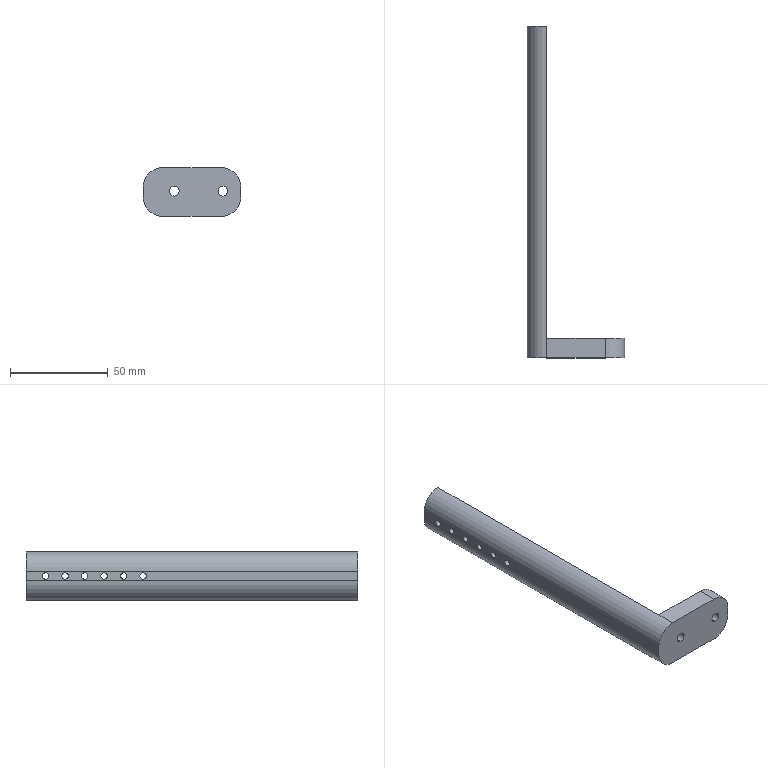Part | STEP file | L.step.STEP.STEP-181.STEP | 1 solid | 28 faces | box 50 x 170 x 25 mm | volume 43868 mm3 | cylinder 20 | plane 8 | commonest cylinder face diameters 3.3 x12 5 x4 20 x4
STEP:
#1=CARTESIAN_POINT('',(96.633,122.7,-36.277));
#2=VERTEX_POINT('',#1);
#3=CARTESIAN_POINT('',(96.633,122.7,-39.577));
#4=VERTEX_POINT('',#3);
#5=CARTESIAN_POINT('',(96.633,122.7,-37.927));
#6=DIRECTION('',(1.,0.,0.));
#7=DIRECTION('',(0.,0.,-1.));
#8=AXIS2_PLACEMENT_3D('',#5,#6,#7);
#9=CIRCLE('',#8,1.65);
#10=EDGE_CURVE('',#2,#4,#9,.T.);
#11=ORIENTED_EDGE('',*,*,#10,.F.);
#12=CARTESIAN_POINT('',(106.633,122.7,-36.277));
#13=VERTEX_POINT('',#12);
#14=CARTESIAN_POINT('',(106.633,122.7,-36.277));
#15=DIRECTION('',(1.,0.,0.));
#16=VECTOR('',#15,1000.);
#17=LINE('',#14,#16);
#18=EDGE_CURVE('',#2,#13,#17,.T.);
#19=ORIENTED_EDGE('',*,*,#18,.T.);
#20=CARTESIAN_POINT('',(106.633,122.7,-39.577));
#21=VERTEX_POINT('',#20);
#22=CARTESIAN_POINT('',(106.633,122.7,-37.927));
#23=DIRECTION('',(1.,0.,0.));
#24=DIRECTION('',(0.,0.,-1.));
#25=AXIS2_PLACEMENT_3D('',#22,#23,#24);
#26=CIRCLE('',#25,1.65);
#27=EDGE_CURVE('',#13,#21,#26,.T.);
#28=ORIENTED_EDGE('',*,*,#27,.T.);
#29=CARTESIAN_POINT('',(106.633,122.7,-39.577));
#30=DIRECTION('',(1.,0.,0.));
#31=VECTOR('',#30,1000.);
#32=LINE('',#29,#31);
#33=EDGE_CURVE('',#4,#21,#32,.T.);
#34=ORIENTED_EDGE('',*,*,#33,.F.);
#35=EDGE_LOOP('',(#11,#19,#28,#34));
#36=FACE_OUTER_BOUND('',#35,.T.);
#37=CARTESIAN_POINT('',(106.633,122.7,-37.927));
#38=DIRECTION('',(1.,0.,0.));
#39=DIRECTION('',(0.,0.,-1.));
#40=AXIS2_PLACEMENT_3D('',#37,#38,#39);
#41=CYLINDRICAL_SURFACE('',#40,1.65);
#42=ADVANCED_FACE('',(#36),#41,.F.);
#43=CARTESIAN_POINT('',(96.633,132.7,-36.277));
#44=VERTEX_POINT('',#43);
#45=CARTESIAN_POINT('',(96.633,132.7,-39.577));
#46=VERTEX_POINT('',#45);
#47=CARTESIAN_POINT('',(96.633,132.7,-37.927));
#48=DIRECTION('',(1.,0.,0.));
#49=DIRECTION('',(0.,0.,-1.));
#50=AXIS2_PLACEMENT_3D('',#47,#48,#49);
#51=CIRCLE('',#50,1.65);
#52=EDGE_CURVE('',#44,#46,#51,.T.);
#53=ORIENTED_EDGE('',*,*,#52,.F.);
#54=CARTESIAN_POINT('',(106.633,132.7,-36.277));
#55=VERTEX_POINT('',#54);
#56=CARTESIAN_POINT('',(106.633,132.7,-36.277));
#57=DIRECTION('',(1.,0.,0.));
#58=VECTOR('',#57,1000.);
#59=LINE('',#56,#58);
#60=EDGE_CURVE('',#44,#55,#59,.T.);
#61=ORIENTED_EDGE('',*,*,#60,.T.);
#62=CARTESIAN_POINT('',(106.633,132.7,-39.577));
#63=VERTEX_POINT('',#62);
#64=CARTESIAN_POINT('',(106.633,132.7,-37.927));
#65=DIRECTION('',(1.,0.,0.));
#66=DIRECTION('',(0.,0.,-1.));
#67=AXIS2_PLACEMENT_3D('',#64,#65,#66);
#68=CIRCLE('',#67,1.65);
#69=EDGE_CURVE('',#55,#63,#68,.T.);
#70=ORIENTED_EDGE('',*,*,#69,.T.);
#71=CARTESIAN_POINT('',(106.633,132.7,-39.577));
#72=DIRECTION('',(1.,0.,0.));
#73=VECTOR('',#72,1000.);
#74=LINE('',#71,#73);
#75=EDGE_CURVE('',#46,#63,#74,.T.);
#76=ORIENTED_EDGE('',*,*,#75,.F.);
#77=EDGE_LOOP('',(#53,#61,#70,#76));
#78=FACE_OUTER_BOUND('',#77,.T.);
#79=CARTESIAN_POINT('',(106.633,132.7,-37.927));
#80=DIRECTION('',(1.,0.,0.));
#81=DIRECTION('',(0.,0.,-1.));
#82=AXIS2_PLACEMENT_3D('',#79,#80,#81);
#83=CYLINDRICAL_SURFACE('',#82,1.65);
#84=ADVANCED_FACE('',(#78),#83,.F.);
#85=CARTESIAN_POINT('',(96.633,142.7,-36.277));
#86=VERTEX_POINT('',#85);
#87=CARTESIAN_POINT('',(96.633,142.7,-39.577));
#88=VERTEX_POINT('',#87);
#89=CARTESIAN_POINT('',(96.633,142.7,-37.927));
#90=DIRECTION('',(1.,0.,0.));
#91=DIRECTION('',(0.,0.,-1.));
#92=AXIS2_PLACEMENT_3D('',#89,#90,#91);
#93=CIRCLE('',#92,1.65);
#94=EDGE_CURVE('',#86,#88,#93,.T.);
#95=ORIENTED_EDGE('',*,*,#94,.F.);
#96=CARTESIAN_POINT('',(106.633,142.7,-36.277));
#97=VERTEX_POINT('',#96);
#98=CARTESIAN_POINT('',(106.633,142.7,-36.277));
#99=DIRECTION('',(1.,0.,0.));
#100=VECTOR('',#99,1000.);
#101=LINE('',#98,#100);
#102=EDGE_CURVE('',#86,#97,#101,.T.);
#103=ORIENTED_EDGE('',*,*,#102,.T.);
#104=CARTESIAN_POINT('',(106.633,142.7,-39.577));
#105=VERTEX_POINT('',#104);
#106=CARTESIAN_POINT('',(106.633,142.7,-37.927));
#107=DIRECTION('',(1.,0.,0.));
#108=DIRECTION('',(0.,0.,-1.));
#109=AXIS2_PLACEMENT_3D('',#106,#107,#108);
#110=CIRCLE('',#109,1.65);
#111=EDGE_CURVE('',#97,#105,#110,.T.);
#112=ORIENTED_EDGE('',*,*,#111,.T.);
#113=CARTESIAN_POINT('',(106.633,142.7,-39.577));
#114=DIRECTION('',(1.,0.,0.));
#115=VECTOR('',#114,1000.);
#116=LINE('',#113,#115);
#117=EDGE_CURVE('',#88,#105,#116,.T.);
#118=ORIENTED_EDGE('',*,*,#117,.F.);
#119=EDGE_LOOP('',(#95,#103,#112,#118));
#120=FACE_OUTER_BOUND('',#119,.T.);
#121=CARTESIAN_POINT('',(106.633,142.7,-37.927));
#122=DIRECTION('',(1.,0.,0.));
#123=DIRECTION('',(0.,0.,-1.));
#124=AXIS2_PLACEMENT_3D('',#121,#122,#123);
#125=CYLINDRICAL_SURFACE('',#124,1.65);
#126=ADVANCED_FACE('',(#120),#125,.F.);
#127=CARTESIAN_POINT('',(96.633,152.7,-36.277));
#128=VERTEX_POINT('',#127);
#129=CARTESIAN_POINT('',(96.633,152.7,-39.577));
#130=VERTEX_POINT('',#129);
#131=CARTESIAN_POINT('',(96.633,152.7,-37.927));
#132=DIRECTION('',(1.,0.,0.));
#133=DIRECTION('',(0.,0.,-1.));
#134=AXIS2_PLACEMENT_3D('',#131,#132,#133);
#135=CIRCLE('',#134,1.65);
#136=EDGE_CURVE('',#128,#130,#135,.T.);
#137=ORIENTED_EDGE('',*,*,#136,.F.);
#138=CARTESIAN_POINT('',(106.633,152.7,-36.277));
#139=VERTEX_POINT('',#138);
#140=CARTESIAN_POINT('',(106.633,152.7,-36.277));
#141=DIRECTION('',(1.,0.,0.));
#142=VECTOR('',#141,1000.);
#143=LINE('',#140,#142);
#144=EDGE_CURVE('',#128,#139,#143,.T.);
#145=ORIENTED_EDGE('',*,*,#144,.T.);
#146=CARTESIAN_POINT('',(106.633,152.7,-39.577));
#147=VERTEX_POINT('',#146);
#148=CARTESIAN_POINT('',(106.633,152.7,-37.927));
#149=DIRECTION('',(1.,0.,0.));
#150=DIRECTION('',(0.,0.,-1.));
#151=AXIS2_PLACEMENT_3D('',#148,#149,#150);
#152=CIRCLE('',#151,1.65);
#153=EDGE_CURVE('',#139,#147,#152,.T.);
#154=ORIENTED_EDGE('',*,*,#153,.T.);
#155=CARTESIAN_POINT('',(106.633,152.7,-39.577));
#156=DIRECTION('',(1.,0.,0.));
#157=VECTOR('',#156,1000.);
#158=LINE('',#155,#157);
#159=EDGE_CURVE('',#130,#147,#158,.T.);
#160=ORIENTED_EDGE('',*,*,#159,.F.);
#161=EDGE_LOOP('',(#137,#145,#154,#160));
#162=FACE_OUTER_BOUND('',#161,.T.);
#163=CARTESIAN_POINT('',(106.633,152.7,-37.927));
#164=DIRECTION('',(1.,0.,0.));
#165=DIRECTION('',(0.,0.,-1.));
#166=AXIS2_PLACEMENT_3D('',#163,#164,#165);
#167=CYLINDRICAL_SURFACE('',#166,1.65);
#168=ADVANCED_FACE('',(#162),#167,.F.);
#169=CARTESIAN_POINT('',(96.633,162.7,-36.277));
#170=VERTEX_POINT('',#169);
#171=CARTESIAN_POINT('',(96.633,162.7,-39.577));
#172=VERTEX_POINT('',#171);
#173=CARTESIAN_POINT('',(96.633,162.7,-37.927));
#174=DIRECTION('',(1.,0.,0.));
#175=DIRECTION('',(0.,0.,-1.));
#176=AXIS2_PLACEMENT_3D('',#173,#174,#175);
#177=CIRCLE('',#176,1.65);
#178=EDGE_CURVE('',#170,#172,#177,.T.);
#179=ORIENTED_EDGE('',*,*,#178,.F.);
#180=CARTESIAN_POINT('',(106.633,162.7,-36.277));
#181=VERTEX_POINT('',#180);
#182=CARTESIAN_POINT('',(106.633,162.7,-36.277));
#183=DIRECTION('',(1.,0.,0.));
#184=VECTOR('',#183,1000.);
#185=LINE('',#182,#184);
#186=EDGE_CURVE('',#170,#181,#185,.T.);
#187=ORIENTED_EDGE('',*,*,#186,.T.);
#188=CARTESIAN_POINT('',(106.633,162.7,-39.577));
#189=VERTEX_POINT('',#188);
#190=CARTESIAN_POINT('',(106.633,162.7,-37.927));
#191=DIRECTION('',(1.,0.,0.));
#192=DIRECTION('',(0.,0.,-1.));
#193=AXIS2_PLACEMENT_3D('',#190,#191,#192);
#194=CIRCLE('',#193,1.65);
#195=EDGE_CURVE('',#181,#189,#194,.T.);
#196=ORIENTED_EDGE('',*,*,#195,.T.);
#197=CARTESIAN_POINT('',(106.633,162.7,-39.577));
#198=DIRECTION('',(1.,0.,0.));
#199=VECTOR('',#198,1000.);
#200=LINE('',#197,#199);
#201=EDGE_CURVE('',#172,#189,#200,.T.);
#202=ORIENTED_EDGE('',*,*,#201,.F.);
#203=EDGE_LOOP('',(#179,#187,#196,#202));
#204=FACE_OUTER_BOUND('',#203,.T.);
#205=CARTESIAN_POINT('',(106.633,162.7,-37.927));
#206=DIRECTION('',(1.,0.,0.));
#207=DIRECTION('',(0.,0.,-1.));
#208=AXIS2_PLACEMENT_3D('',#205,#206,#207);
#209=CYLINDRICAL_SURFACE('',#208,1.65);
#210=ADVANCED_FACE('',(#204),#209,.F.);
#211=CARTESIAN_POINT('',(96.633,172.7,-36.277));
#212=VERTEX_POINT('',#211);
#213=CARTESIAN_POINT('',(96.633,172.7,-39.577));
#214=VERTEX_POINT('',#213);
#215=CARTESIAN_POINT('',(96.633,172.7,-37.927));
#216=DIRECTION('',(1.,0.,0.));
#217=DIRECTION('',(0.,0.,-1.));
#218=AXIS2_PLACEMENT_3D('',#215,#216,#217);
#219=CIRCLE('',#218,1.65);
#220=EDGE_CURVE('',#212,#214,#219,.T.);
#221=ORIENTED_EDGE('',*,*,#220,.F.);
#222=CARTESIAN_POINT('',(106.633,172.7,-36.277));
#223=VERTEX_POINT('',#222);
#224=CARTESIAN_POINT('',(106.633,172.7,-36.277));
#225=DIRECTION('',(1.,0.,0.));
#226=VECTOR('',#225,1000.);
#227=LINE('',#224,#226);
#228=EDGE_CURVE('',#212,#223,#227,.T.);
#229=ORIENTED_EDGE('',*,*,#228,.T.);
#230=CARTESIAN_POINT('',(106.633,172.7,-39.577));
#231=VERTEX_POINT('',#230);
#232=CARTESIAN_POINT('',(106.633,172.7,-37.927));
#233=DIRECTION('',(1.,0.,0.));
#234=DIRECTION('',(0.,0.,-1.));
#235=AXIS2_PLACEMENT_3D('',#232,#233,#234);
#236=CIRCLE('',#235,1.65);
#237=EDGE_CURVE('',#223,#231,#236,.T.);
#238=ORIENTED_EDGE('',*,*,#237,.T.);
#239=CARTESIAN_POINT('',(106.633,172.7,-39.577));
#240=DIRECTION('',(1.,0.,0.));
#241=VECTOR('',#240,1000.);
#242=LINE('',#239,#241);
#243=EDGE_CURVE('',#214,#231,#242,.T.);
#244=ORIENTED_EDGE('',*,*,#243,.F.);
#245=EDGE_LOOP('',(#221,#229,#238,#244));
#246=FACE_OUTER_BOUND('',#245,.T.);
#247=CARTESIAN_POINT('',(106.633,172.7,-37.927));
#248=DIRECTION('',(1.,0.,0.));
#249=DIRECTION('',(0.,0.,-1.));
#250=AXIS2_PLACEMENT_3D('',#247,#248,#249);
#251=CYLINDRICAL_SURFACE('',#250,1.65);
#252=ADVANCED_FACE('',(#246),#251,.F.);
#253=CARTESIAN_POINT('',(112.5,22.7,-35.));
#254=VERTEX_POINT('',#253);
#255=CARTESIAN_POINT('',(112.5,22.7,-40.));
#256=VERTEX_POINT('',#255);
#257=CARTESIAN_POINT('',(112.5,22.7,-37.5));
#258=DIRECTION('',(0.,-1.,0.));
#259=DIRECTION('',(0.,0.,-1.));
#260=AXIS2_PLACEMENT_3D('',#257,#258,#259);
#261=CIRCLE('',#260,2.5);
#262=EDGE_CURVE('',#254,#256,#261,.T.);
#263=ORIENTED_EDGE('',*,*,#262,.F.);
#264=CARTESIAN_POINT('',(112.5,12.7,-35.));
#265=VERTEX_POINT('',#264);
#266=CARTESIAN_POINT('',(112.5,0.,-35.));
#267=DIRECTION('',(0.,-1.,0.));
#268=VECTOR('',#267,1000.);
#269=LINE('',#266,#268);
#270=EDGE_CURVE('',#254,#265,#269,.T.);
#271=ORIENTED_EDGE('',*,*,#270,.T.);
#272=CARTESIAN_POINT('',(112.5,12.7,-40.));
#273=VERTEX_POINT('',#272);
#274=CARTESIAN_POINT('',(112.5,12.7,-37.5));
#275=DIRECTION('',(0.,1.,0.));
#276=DIRECTION('',(0.,0.,1.));
#277=AXIS2_PLACEMENT_3D('',#274,#275,#276);
#278=CIRCLE('',#277,2.5);
#279=EDGE_CURVE('',#273,#265,#278,.T.);
#280=ORIENTED_EDGE('',*,*,#279,.F.);
#281=CARTESIAN_POINT('',(112.5,0.,-40.));
#282=DIRECTION('',(0.,-1.,0.));
#283=VECTOR('',#282,1000.);
#284=LINE('',#281,#283);
#285=EDGE_CURVE('',#256,#273,#284,.T.);
#286=ORIENTED_EDGE('',*,*,#285,.F.);
#287=EDGE_LOOP('',(#263,#271,#280,#286));
#288=FACE_OUTER_BOUND('',#287,.T.);
#289=CARTESIAN_POINT('',(112.5,0.,-37.5));
#290=DIRECTION('',(0.,-1.,0.));
#291=DIRECTION('',(0.,0.,-1.));
#292=AXIS2_PLACEMENT_3D('',#289,#290,#291);
#293=CYLINDRICAL_SURFACE('',#292,2.5);
#294=ADVANCED_FACE('',(#288),#293,.F.);
#295=CARTESIAN_POINT('',(137.5,22.7,-35.));
#296=VERTEX_POINT('',#295);
#297=CARTESIAN_POINT('',(137.5,22.7,-40.));
#298=VERTEX_POINT('',#297);
#299=CARTESIAN_POINT('',(137.5,22.7,-37.5));
#300=DIRECTION('',(0.,-1.,0.));
#301=DIRECTION('',(0.,0.,-1.));
#302=AXIS2_PLACEMENT_3D('',#299,#300,#301);
#303=CIRCLE('',#302,2.5);
#304=EDGE_CURVE('',#296,#298,#303,.T.);
#305=ORIENTED_EDGE('',*,*,#304,.F.);
#306=CARTESIAN_POINT('',(137.5,12.7,-35.));
#307=VERTEX_POINT('',#306);
#308=CARTESIAN_POINT('',(137.5,0.,-35.));
#309=DIRECTION('',(0.,-1.,0.));
#310=VECTOR('',#309,1000.);
#311=LINE('',#308,#310);
#312=EDGE_CURVE('',#296,#307,#311,.T.);
#313=ORIENTED_EDGE('',*,*,#312,.T.);
#314=CARTESIAN_POINT('',(137.5,12.7,-40.));
#315=VERTEX_POINT('',#314);
#316=CARTESIAN_POINT('',(137.5,12.7,-37.5));
#317=DIRECTION('',(0.,1.,0.));
#318=DIRECTION('',(0.,0.,1.));
#319=AXIS2_PLACEMENT_3D('',#316,#317,#318);
#320=CIRCLE('',#319,2.5);
#321=EDGE_CURVE('',#315,#307,#320,.T.);
#322=ORIENTED_EDGE('',*,*,#321,.F.);
#323=CARTESIAN_POINT('',(137.5,0.,-40.));
#324=DIRECTION('',(0.,-1.,0.));
#325=VECTOR('',#324,1000.);
#326=LINE('',#323,#325);
#327=EDGE_CURVE('',#298,#315,#326,.T.);
#328=ORIENTED_EDGE('',*,*,#327,.F.);
#329=EDGE_LOOP('',(#305,#313,#322,#328));
#330=FACE_OUTER_BOUND('',#329,.T.);
#331=CARTESIAN_POINT('',(137.5,0.,-37.5));
#332=DIRECTION('',(0.,-1.,0.));
#333=DIRECTION('',(0.,0.,-1.));
#334=AXIS2_PLACEMENT_3D('',#331,#332,#333);
#335=CYLINDRICAL_SURFACE('',#334,2.5);
#336=ADVANCED_FACE('',(#330),#335,.F.);
#337=CARTESIAN_POINT('',(112.5,22.7,-37.5));
#338=DIRECTION('',(0.,-1.,0.));
#339=DIRECTION('',(0.,0.,-1.));
#340=AXIS2_PLACEMENT_3D('',#337,#338,#339);
#341=CIRCLE('',#340,2.5);
#342=EDGE_CURVE('',#256,#254,#341,.T.);
#343=ORIENTED_EDGE('',*,*,#342,.T.);
#344=ORIENTED_EDGE('',*,*,#262,.T.);
#345=EDGE_LOOP('',(#343,#344));
#346=FACE_BOUND('',#345,.T.);
#347=CARTESIAN_POINT('',(137.5,22.7,-37.5));
#348=DIRECTION('',(0.,-1.,0.));
#349=DIRECTION('',(0.,0.,-1.));
#350=AXIS2_PLACEMENT_3D('',#347,#348,#349);
#351=CIRCLE('',#350,2.5);
#352=EDGE_CURVE('',#298,#296,#351,.T.);
#353=ORIENTED_EDGE('',*,*,#352,.T.);
#354=ORIENTED_EDGE('',*,*,#304,.T.);
#355=EDGE_LOOP('',(#353,#354));
#356=FACE_BOUND('',#355,.T.);
#357=CARTESIAN_POINT('',(136.633,22.7,-50.427));
#358=VERTEX_POINT('',#357);
#359=CARTESIAN_POINT('',(106.633,22.7,-50.427));
#360=VERTEX_POINT('',#359);
#361=CARTESIAN_POINT('',(106.633,22.7,-50.427));
#362=DIRECTION('',(-1.,0.,0.));
#363=VECTOR('',#362,1000.);
#364=LINE('',#361,#363);
#365=EDGE_CURVE('',#358,#360,#364,.T.);
#366=ORIENTED_EDGE('',*,*,#365,.T.);
#367=CARTESIAN_POINT('',(106.633,22.7,-25.427));
#368=VERTEX_POINT('',#367);
#369=CARTESIAN_POINT('',(106.633,22.7,0.));
#370=DIRECTION('',(0.,0.,1.));
#371=VECTOR('',#370,1000.);
#372=LINE('',#369,#371);
#373=EDGE_CURVE('',#360,#368,#372,.T.);
#374=ORIENTED_EDGE('',*,*,#373,.T.);
#375=CARTESIAN_POINT('',(136.633,22.7,-25.427));
#376=VERTEX_POINT('',#375);
#377=CARTESIAN_POINT('',(106.633,22.7,-25.427));
#378=DIRECTION('',(1.,0.,0.));
#379=VECTOR('',#378,1000.);
#380=LINE('',#377,#379);
#381=EDGE_CURVE('',#368,#376,#380,.T.);
#382=ORIENTED_EDGE('',*,*,#381,.T.);
#383=CARTESIAN_POINT('',(146.633,22.7,-35.427));
#384=VERTEX_POINT('',#383);
#385=CARTESIAN_POINT('',(136.633,22.7,-35.427));
#386=DIRECTION('',(0.,1.,0.));
#387=DIRECTION('',(0.,0.,1.));
#388=AXIS2_PLACEMENT_3D('',#385,#386,#387);
#389=CIRCLE('',#388,10.);
#390=EDGE_CURVE('',#376,#384,#389,.T.);
#391=ORIENTED_EDGE('',*,*,#390,.T.);
#392=CARTESIAN_POINT('',(146.633,22.7,-40.427));
#393=VERTEX_POINT('',#392);
#394=CARTESIAN_POINT('',(146.633,22.7,-40.427));
#395=DIRECTION('',(0.,0.,-1.));
#396=VECTOR('',#395,1000.);
#397=LINE('',#394,#396);
#398=EDGE_CURVE('',#384,#393,#397,.T.);
#399=ORIENTED_EDGE('',*,*,#398,.T.);
#400=CARTESIAN_POINT('',(136.633,22.7,-40.427));
#401=DIRECTION('',(0.,1.,0.));
#402=DIRECTION('',(0.,0.,1.));
#403=AXIS2_PLACEMENT_3D('',#400,#401,#402);
#404=CIRCLE('',#403,10.);
#405=EDGE_CURVE('',#393,#358,#404,.T.);
#406=ORIENTED_EDGE('',*,*,#405,.T.);
#407=EDGE_LOOP('',(#366,#374,#382,#391,#399,#406));
#408=FACE_OUTER_BOUND('',#407,.T.);
#409=CARTESIAN_POINT('',(136.633,22.7,-40.427));
#410=DIRECTION('',(0.,1.,0.));
#411=DIRECTION('',(1.,0.,0.));
#412=AXIS2_PLACEMENT_3D('',#409,#410,#411);
#413=PLANE('',#412);
#414=ADVANCED_FACE('',(#346,#356,#408),#413,.T.);
#415=ORIENTED_EDGE('',*,*,#279,.T.);
#416=CARTESIAN_POINT('',(112.5,12.7,-37.5));
#417=DIRECTION('',(0.,1.,0.));
#418=DIRECTION('',(0.,0.,1.));
#419=AXIS2_PLACEMENT_3D('',#416,#417,#418);
#420=CIRCLE('',#419,2.5);
#421=EDGE_CURVE('',#265,#273,#420,.T.);
#422=ORIENTED_EDGE('',*,*,#421,.T.);
#423=EDGE_LOOP('',(#415,#422));
#424=FACE_BOUND('',#423,.T.);
#425=ORIENTED_EDGE('',*,*,#321,.T.);
#426=CARTESIAN_POINT('',(137.5,12.7,-37.5));
#427=DIRECTION('',(0.,1.,0.));
#428=DIRECTION('',(0.,0.,1.));
#429=AXIS2_PLACEMENT_3D('',#426,#427,#428);
#430=CIRCLE('',#429,2.5);
#431=EDGE_CURVE('',#307,#315,#430,.T.);
#432=ORIENTED_EDGE('',*,*,#431,.T.);
#433=EDGE_LOOP('',(#425,#432));
#434=FACE_BOUND('',#433,.T.);
#435=CARTESIAN_POINT('',(146.633,12.7,-35.427));
#436=VERTEX_POINT('',#435);
#437=CARTESIAN_POINT('',(146.633,12.7,-40.427));
#438=VERTEX_POINT('',#437);
#439=CARTESIAN_POINT('',(146.633,12.7,-40.427));
#440=DIRECTION('',(0.,0.,-1.));
#441=VECTOR('',#440,1000.);
#442=LINE('',#439,#441);
#443=EDGE_CURVE('',#436,#438,#442,.T.);
#444=ORIENTED_EDGE('',*,*,#443,.F.);
#445=CARTESIAN_POINT('',(136.633,12.7,-25.427));
#446=VERTEX_POINT('',#445);
#447=CARTESIAN_POINT('',(136.633,12.7,-35.427));
#448=DIRECTION('',(0.,1.,0.));
#449=DIRECTION('',(0.,0.,1.));
#450=AXIS2_PLACEMENT_3D('',#447,#448,#449);
#451=CIRCLE('',#450,10.);
#452=EDGE_CURVE('',#446,#436,#451,.T.);
#453=ORIENTED_EDGE('',*,*,#452,.F.);
#454=CARTESIAN_POINT('',(106.633,12.7,-25.427));
#455=VERTEX_POINT('',#454);
#456=CARTESIAN_POINT('',(106.633,12.7,-25.427));
#457=DIRECTION('',(1.,0.,0.));
#458=VECTOR('',#457,1000.);
#459=LINE('',#456,#458);
#460=EDGE_CURVE('',#455,#446,#459,.T.);
#461=ORIENTED_EDGE('',*,*,#460,.F.);
#462=CARTESIAN_POINT('',(96.633,12.7,-35.427));
#463=VERTEX_POINT('',#462);
#464=CARTESIAN_POINT('',(106.633,12.7,-35.427));
#465=DIRECTION('',(0.,1.,0.));
#466=DIRECTION('',(0.,0.,-1.));
#467=AXIS2_PLACEMENT_3D('',#464,#465,#466);
#468=CIRCLE('',#467,10.);
#469=EDGE_CURVE('',#463,#455,#468,.T.);
#470=ORIENTED_EDGE('',*,*,#469,.F.);
#471=CARTESIAN_POINT('',(96.633,12.7,-40.427));
#472=VERTEX_POINT('',#471);
#473=CARTESIAN_POINT('',(96.633,12.7,-40.427));
#474=DIRECTION('',(0.,0.,1.));
#475=VECTOR('',#474,1000.);
#476=LINE('',#473,#475);
#477=EDGE_CURVE('',#472,#463,#476,.T.);
#478=ORIENTED_EDGE('',*,*,#477,.F.);
#479=CARTESIAN_POINT('',(106.633,12.7,-50.427));
#480=VERTEX_POINT('',#479);
#481=CARTESIAN_POINT('',(106.633,12.7,-40.427));
#482=DIRECTION('',(0.,1.,0.));
#483=DIRECTION('',(0.,0.,-1.));
#484=AXIS2_PLACEMENT_3D('',#481,#482,#483);
#485=CIRCLE('',#484,10.);
#486=EDGE_CURVE('',#480,#472,#485,.T.);
#487=ORIENTED_EDGE('',*,*,#486,.F.);
#488=CARTESIAN_POINT('',(136.633,12.7,-50.427));
#489=VERTEX_POINT('',#488);
#490=CARTESIAN_POINT('',(106.633,12.7,-50.427));
#491=DIRECTION('',(-1.,0.,0.));
#492=VECTOR('',#491,1000.);
#493=LINE('',#490,#492);
#494=EDGE_CURVE('',#489,#480,#493,.T.);
#495=ORIENTED_EDGE('',*,*,#494,.F.);
#496=CARTESIAN_POINT('',(136.633,12.7,-40.427));
#497=DIRECTION('',(0.,1.,0.));
#498=DIRECTION('',(0.,0.,1.));
#499=AXIS2_PLACEMENT_3D('',#496,#497,#498);
#500=CIRCLE('',#499,10.);
#501=EDGE_CURVE('',#438,#489,#500,.T.);
#502=ORIENTED_EDGE('',*,*,#501,.F.);
#503=EDGE_LOOP('',(#444,#453,#461,#470,#478,#487,#495,#502));
#504=FACE_OUTER_BOUND('',#503,.T.);
#505=CARTESIAN_POINT('',(136.633,12.7,-40.427));
#506=DIRECTION('',(0.,1.,0.));
#507=DIRECTION('',(1.,0.,0.));
#508=AXIS2_PLACEMENT_3D('',#505,#506,#507);
#509=PLANE('',#508);
#510=ADVANCED_FACE('',(#424,#434,#504),#509,.F.);
#511=ORIENTED_EDGE('',*,*,#501,.T.);
#512=CARTESIAN_POINT('',(136.633,22.7,-50.427));
#513=DIRECTION('',(0.,-1.,0.));
#514=VECTOR('',#513,1000.);
#515=LINE('',#512,#514);
#516=EDGE_CURVE('',#358,#489,#515,.T.);
#517=ORIENTED_EDGE('',*,*,#516,.F.);
#518=ORIENTED_EDGE('',*,*,#405,.F.);
#519=CARTESIAN_POINT('',(146.633,22.7,-40.427));
#520=DIRECTION('',(0.,-1.,0.));
#521=VECTOR('',#520,1000.);
#522=LINE('',#519,#521);
#523=EDGE_CURVE('',#393,#438,#522,.T.);
#524=ORIENTED_EDGE('',*,*,#523,.T.);
#525=EDGE_LOOP('',(#511,#517,#518,#524));
#526=FACE_OUTER_BOUND('',#525,.T.);
#527=CARTESIAN_POINT('',(136.633,22.7,-40.427));
#528=DIRECTION('',(0.,-1.,0.));
#529=DIRECTION('',(0.,0.,-1.));
#530=AXIS2_PLACEMENT_3D('',#527,#528,#529);
#531=CYLINDRICAL_SURFACE('',#530,10.);
#532=ADVANCED_FACE('',(#526),#531,.T.);
#533=ORIENTED_EDGE('',*,*,#494,.T.);
#534=CARTESIAN_POINT('',(106.633,22.7,-50.427));
#535=DIRECTION('',(0.,-1.,0.));
#536=VECTOR('',#535,1000.);
#537=LINE('',#534,#536);
#538=EDGE_CURVE('',#360,#480,#537,.T.);
#539=ORIENTED_EDGE('',*,*,#538,.F.);
#540=ORIENTED_EDGE('',*,*,#365,.F.);
#541=ORIENTED_EDGE('',*,*,#516,.T.);
#542=EDGE_LOOP('',(#533,#539,#540,#541));
#543=FACE_OUTER_BOUND('',#542,.T.);
#544=CARTESIAN_POINT('',(106.633,22.7,-50.427));
#545=DIRECTION('',(0.,0.,1.));
#546=DIRECTION('',(1.,0.,0.));
#547=AXIS2_PLACEMENT_3D('',#544,#545,#546);
#548=PLANE('',#547);
#549=ADVANCED_FACE('',(#543),#548,.F.);
#550=ORIENTED_EDGE('',*,*,#486,.T.);
#551=CARTESIAN_POINT('',(96.633,182.7,-40.427));
#552=VERTEX_POINT('',#551);
#553=CARTESIAN_POINT('',(96.633,22.7,-40.427));
#554=DIRECTION('',(0.,-1.,0.));
#555=VECTOR('',#554,1000.);
#556=LINE('',#553,#555);
#557=EDGE_CURVE('',#552,#472,#556,.T.);
#558=ORIENTED_EDGE('',*,*,#557,.F.);
#559=CARTESIAN_POINT('',(106.633,182.7,-50.427));
#560=VERTEX_POINT('',#559);
#561=CARTESIAN_POINT('',(106.633,182.7,-40.427));
#562=DIRECTION('',(0.,1.,0.));
#563=DIRECTION('',(0.,0.,1.));
#564=AXIS2_PLACEMENT_3D('',#561,#562,#563);
#565=CIRCLE('',#564,10.);
#566=EDGE_CURVE('',#560,#552,#565,.T.);
#567=ORIENTED_EDGE('',*,*,#566,.F.);
#568=CARTESIAN_POINT('',(106.633,182.7,-50.427));
#569=DIRECTION('',(0.,-1.,0.));
#570=VECTOR('',#569,1000.);
#571=LINE('',#568,#570);
#572=EDGE_CURVE('',#560,#360,#571,.T.);
#573=ORIENTED_EDGE('',*,*,#572,.T.);
#574=ORIENTED_EDGE('',*,*,#538,.T.);
#575=EDGE_LOOP('',(#550,#558,#567,#573,#574));
#576=FACE_OUTER_BOUND('',#575,.T.);
#577=CARTESIAN_POINT('',(106.633,22.7,-40.427));
#578=DIRECTION('',(0.,-1.,0.));
#579=DIRECTION('',(0.,0.,-1.));
#580=AXIS2_PLACEMENT_3D('',#577,#578,#579);
#581=CYLINDRICAL_SURFACE('',#580,10.);
#582=ADVANCED_FACE('',(#576),#581,.T.);
#583=CARTESIAN_POINT('',(96.633,122.7,-37.927));
#584=DIRECTION('',(1.,0.,0.));
#585=DIRECTION('',(0.,0.,-1.));
#586=AXIS2_PLACEMENT_3D('',#583,#584,#585);
#587=CIRCLE('',#586,1.65);
#588=EDGE_CURVE('',#4,#2,#587,.T.);
#589=ORIENTED_EDGE('',*,*,#588,.T.);
#590=ORIENTED_EDGE('',*,*,#10,.T.);
#591=EDGE_LOOP('',(#589,#590));
#592=FACE_BOUND('',#591,.T.);
#593=CARTESIAN_POINT('',(96.633,132.7,-37.927));
#594=DIRECTION('',(1.,0.,0.));
#595=DIRECTION('',(0.,0.,-1.));
#596=AXIS2_PLACEMENT_3D('',#593,#594,#595);
#597=CIRCLE('',#596,1.65);
#598=EDGE_CURVE('',#46,#44,#597,.T.);
#599=ORIENTED_EDGE('',*,*,#598,.T.);
#600=ORIENTED_EDGE('',*,*,#52,.T.);
#601=EDGE_LOOP('',(#599,#600));
#602=FACE_BOUND('',#601,.T.);
#603=CARTESIAN_POINT('',(96.633,142.7,-37.927));
#604=DIRECTION('',(1.,0.,0.));
#605=DIRECTION('',(0.,0.,-1.));
#606=AXIS2_PLACEMENT_3D('',#603,#604,#605);
#607=CIRCLE('',#606,1.65);
#608=EDGE_CURVE('',#88,#86,#607,.T.);
#609=ORIENTED_EDGE('',*,*,#608,.T.);
#610=ORIENTED_EDGE('',*,*,#94,.T.);
#611=EDGE_LOOP('',(#609,#610));
#612=FACE_BOUND('',#611,.T.);
#613=CARTESIAN_POINT('',(96.633,152.7,-37.927));
#614=DIRECTION('',(1.,0.,0.));
#615=DIRECTION('',(0.,0.,-1.));
#616=AXIS2_PLACEMENT_3D('',#613,#614,#615);
#617=CIRCLE('',#616,1.65);
#618=EDGE_CURVE('',#130,#128,#617,.T.);
#619=ORIENTED_EDGE('',*,*,#618,.T.);
#620=ORIENTED_EDGE('',*,*,#136,.T.);
#621=EDGE_LOOP('',(#619,#620));
#622=FACE_BOUND('',#621,.T.);
#623=CARTESIAN_POINT('',(96.633,162.7,-37.927));
#624=DIRECTION('',(1.,0.,0.));
#625=DIRECTION('',(0.,0.,-1.));
#626=AXIS2_PLACEMENT_3D('',#623,#624,#625);
#627=CIRCLE('',#626,1.65);
#628=EDGE_CURVE('',#172,#170,#627,.T.);
#629=ORIENTED_EDGE('',*,*,#628,.T.);
#630=ORIENTED_EDGE('',*,*,#178,.T.);
#631=EDGE_LOOP('',(#629,#630));
#632=FACE_BOUND('',#631,.T.);
#633=CARTESIAN_POINT('',(96.633,172.7,-37.927));
#634=DIRECTION('',(1.,0.,0.));
#635=DIRECTION('',(0.,0.,-1.));
#636=AXIS2_PLACEMENT_3D('',#633,#634,#635);
#637=CIRCLE('',#636,1.65);
#638=EDGE_CURVE('',#214,#212,#637,.T.);
#639=ORIENTED_EDGE('',*,*,#638,.T.);
#640=ORIENTED_EDGE('',*,*,#220,.T.);
#641=EDGE_LOOP('',(#639,#640));
#642=FACE_BOUND('',#641,.T.);
#643=ORIENTED_EDGE('',*,*,#477,.T.);
#644=CARTESIAN_POINT('',(96.633,182.7,-35.427));
#645=VERTEX_POINT('',#644);
#646=CARTESIAN_POINT('',(96.633,22.7,-35.427));
#647=DIRECTION('',(0.,-1.,0.));
#648=VECTOR('',#647,1000.);
#649=LINE('',#646,#648);
#650=EDGE_CURVE('',#645,#463,#649,.T.);
#651=ORIENTED_EDGE('',*,*,#650,.F.);
#652=CARTESIAN_POINT('',(96.633,182.7,0.));
#653=DIRECTION('',(0.,0.,1.));
#654=VECTOR('',#653,1000.);
#655=LINE('',#652,#654);
#656=EDGE_CURVE('',#552,#645,#655,.T.);
#657=ORIENTED_EDGE('',*,*,#656,.F.);
#658=ORIENTED_EDGE('',*,*,#557,.T.);
#659=EDGE_LOOP('',(#643,#651,#657,#658));
#660=FACE_OUTER_BOUND('',#659,.T.);
#661=CARTESIAN_POINT('',(96.633,22.7,-40.427));
#662=DIRECTION('',(1.,0.,0.));
#663=DIRECTION('',(0.,1.,0.));
#664=AXIS2_PLACEMENT_3D('',#661,#662,#663);
#665=PLANE('',#664);
#666=ADVANCED_FACE('',(#592,#602,#612,#622,#632,#642,#660),#665,.F.);
#667=ORIENTED_EDGE('',*,*,#469,.T.);
#668=CARTESIAN_POINT('',(106.633,22.7,-25.427));
#669=DIRECTION('',(0.,-1.,0.));
#670=VECTOR('',#669,1000.);
#671=LINE('',#668,#670);
#672=EDGE_CURVE('',#368,#455,#671,.T.);
#673=ORIENTED_EDGE('',*,*,#672,.F.);
#674=CARTESIAN_POINT('',(106.633,182.7,-25.427));
#675=VERTEX_POINT('',#674);
#676=CARTESIAN_POINT('',(106.633,182.7,-25.427));
#677=DIRECTION('',(0.,-1.,0.));
#678=VECTOR('',#677,1000.);
#679=LINE('',#676,#678);
#680=EDGE_CURVE('',#675,#368,#679,.T.);
#681=ORIENTED_EDGE('',*,*,#680,.F.);
#682=CARTESIAN_POINT('',(106.633,182.7,-35.427));
#683=DIRECTION('',(0.,1.,0.));
#684=DIRECTION('',(0.,0.,1.));
#685=AXIS2_PLACEMENT_3D('',#682,#683,#684);
#686=CIRCLE('',#685,10.);
#687=EDGE_CURVE('',#645,#675,#686,.T.);
#688=ORIENTED_EDGE('',*,*,#687,.F.);
#689=ORIENTED_EDGE('',*,*,#650,.T.);
#690=EDGE_LOOP('',(#667,#673,#681,#688,#689));
#691=FACE_OUTER_BOUND('',#690,.T.);
#692=CARTESIAN_POINT('',(106.633,22.7,-35.427));
#693=DIRECTION('',(0.,-1.,0.));
#694=DIRECTION('',(0.,0.,-1.));
#695=AXIS2_PLACEMENT_3D('',#692,#693,#694);
#696=CYLINDRICAL_SURFACE('',#695,10.);
#697=ADVANCED_FACE('',(#691),#696,.T.);
#698=ORIENTED_EDGE('',*,*,#460,.T.);
#699=CARTESIAN_POINT('',(136.633,22.7,-25.427));
#700=DIRECTION('',(0.,-1.,0.));
#701=VECTOR('',#700,1000.);
#702=LINE('',#699,#701);
#703=EDGE_CURVE('',#376,#446,#702,.T.);
#704=ORIENTED_EDGE('',*,*,#703,.F.);
#705=ORIENTED_EDGE('',*,*,#381,.F.);
#706=ORIENTED_EDGE('',*,*,#672,.T.);
#707=EDGE_LOOP('',(#698,#704,#705,#706));
#708=FACE_OUTER_BOUND('',#707,.T.);
#709=CARTESIAN_POINT('',(106.633,22.7,-25.427));
#710=DIRECTION('',(0.,0.,-1.));
#711=DIRECTION('',(0.,-1.,0.));
#712=AXIS2_PLACEMENT_3D('',#709,#710,#711);
#713=PLANE('',#712);
#714=ADVANCED_FACE('',(#708),#713,.F.);
#715=ORIENTED_EDGE('',*,*,#452,.T.);
#716=CARTESIAN_POINT('',(146.633,22.7,-35.427));
#717=DIRECTION('',(0.,-1.,0.));
#718=VECTOR('',#717,1000.);
#719=LINE('',#716,#718);
#720=EDGE_CURVE('',#384,#436,#719,.T.);
#721=ORIENTED_EDGE('',*,*,#720,.F.);
#722=ORIENTED_EDGE('',*,*,#390,.F.);
#723=ORIENTED_EDGE('',*,*,#703,.T.);
#724=EDGE_LOOP('',(#715,#721,#722,#723));
#725=FACE_OUTER_BOUND('',#724,.T.);
#726=CARTESIAN_POINT('',(136.633,22.7,-35.427));
#727=DIRECTION('',(0.,-1.,0.));
#728=DIRECTION('',(0.,0.,-1.));
#729=AXIS2_PLACEMENT_3D('',#726,#727,#728);
#730=CYLINDRICAL_SURFACE('',#729,10.);
#731=ADVANCED_FACE('',(#725),#730,.T.);
#732=ORIENTED_EDGE('',*,*,#443,.T.);
#733=ORIENTED_EDGE('',*,*,#523,.F.);
#734=ORIENTED_EDGE('',*,*,#398,.F.);
#735=ORIENTED_EDGE('',*,*,#720,.T.);
#736=EDGE_LOOP('',(#732,#733,#734,#735));
#737=FACE_OUTER_BOUND('',#736,.T.);
#738=CARTESIAN_POINT('',(146.633,22.7,-40.427));
#739=DIRECTION('',(-1.,0.,0.));
#740=DIRECTION('',(0.,0.,1.));
#741=AXIS2_PLACEMENT_3D('',#738,#739,#740);
#742=PLANE('',#741);
#743=ADVANCED_FACE('',(#737),#742,.F.);
#744=ORIENTED_EDGE('',*,*,#312,.F.);
#745=ORIENTED_EDGE('',*,*,#352,.F.);
#746=ORIENTED_EDGE('',*,*,#327,.T.);
#747=ORIENTED_EDGE('',*,*,#431,.F.);
#748=EDGE_LOOP('',(#744,#745,#746,#747));
#749=FACE_OUTER_BOUND('',#748,.T.);
#750=CARTESIAN_POINT('',(137.5,0.,-37.5));
#751=DIRECTION('',(0.,-1.,0.));
#752=DIRECTION('',(0.,0.,-1.));
#753=AXIS2_PLACEMENT_3D('',#750,#751,#752);
#754=CYLINDRICAL_SURFACE('',#753,2.5);
#755=ADVANCED_FACE('',(#749),#754,.F.);
#756=ORIENTED_EDGE('',*,*,#270,.F.);
#757=ORIENTED_EDGE('',*,*,#342,.F.);
#758=ORIENTED_EDGE('',*,*,#285,.T.);
#759=ORIENTED_EDGE('',*,*,#421,.F.);
#760=EDGE_LOOP('',(#756,#757,#758,#759));
#761=FACE_OUTER_BOUND('',#760,.T.);
#762=CARTESIAN_POINT('',(112.5,0.,-37.5));
#763=DIRECTION('',(0.,-1.,0.));
#764=DIRECTION('',(0.,0.,-1.));
#765=AXIS2_PLACEMENT_3D('',#762,#763,#764);
#766=CYLINDRICAL_SURFACE('',#765,2.5);
#767=ADVANCED_FACE('',(#761),#766,.F.);
#768=CARTESIAN_POINT('',(106.633,122.7,-37.927));
#769=DIRECTION('',(1.,0.,0.));
#770=DIRECTION('',(0.,0.,-1.));
#771=AXIS2_PLACEMENT_3D('',#768,#769,#770);
#772=CIRCLE('',#771,1.65);
#773=EDGE_CURVE('',#21,#13,#772,.T.);
#774=ORIENTED_EDGE('',*,*,#773,.F.);
#775=ORIENTED_EDGE('',*,*,#27,.F.);
#776=EDGE_LOOP('',(#774,#775));
#777=FACE_BOUND('',#776,.T.);
#778=CARTESIAN_POINT('',(106.633,132.7,-37.927));
#779=DIRECTION('',(1.,0.,0.));
#780=DIRECTION('',(0.,0.,-1.));
#781=AXIS2_PLACEMENT_3D('',#778,#779,#780);
#782=CIRCLE('',#781,1.65);
#783=EDGE_CURVE('',#63,#55,#782,.T.);
#784=ORIENTED_EDGE('',*,*,#783,.F.);
#785=ORIENTED_EDGE('',*,*,#69,.F.);
#786=EDGE_LOOP('',(#784,#785));
#787=FACE_BOUND('',#786,.T.);
#788=CARTESIAN_POINT('',(106.633,142.7,-37.927));
#789=DIRECTION('',(1.,0.,0.));
#790=DIRECTION('',(0.,0.,-1.));
#791=AXIS2_PLACEMENT_3D('',#788,#789,#790);
#792=CIRCLE('',#791,1.65);
#793=EDGE_CURVE('',#105,#97,#792,.T.);
#794=ORIENTED_EDGE('',*,*,#793,.F.);
#795=ORIENTED_EDGE('',*,*,#111,.F.);
#796=EDGE_LOOP('',(#794,#795));
#797=FACE_BOUND('',#796,.T.);
#798=CARTESIAN_POINT('',(106.633,152.7,-37.927));
#799=DIRECTION('',(1.,0.,0.));
#800=DIRECTION('',(0.,0.,-1.));
#801=AXIS2_PLACEMENT_3D('',#798,#799,#800);
#802=CIRCLE('',#801,1.65);
#803=EDGE_CURVE('',#147,#139,#802,.T.);
#804=ORIENTED_EDGE('',*,*,#803,.F.);
#805=ORIENTED_EDGE('',*,*,#153,.F.);
#806=EDGE_LOOP('',(#804,#805));
#807=FACE_BOUND('',#806,.T.);
#808=CARTESIAN_POINT('',(106.633,162.7,-37.927));
#809=DIRECTION('',(1.,0.,0.));
#810=DIRECTION('',(0.,0.,-1.));
#811=AXIS2_PLACEMENT_3D('',#808,#809,#810);
#812=CIRCLE('',#811,1.65);
#813=EDGE_CURVE('',#189,#181,#812,.T.);
#814=ORIENTED_EDGE('',*,*,#813,.F.);
#815=ORIENTED_EDGE('',*,*,#195,.F.);
#816=EDGE_LOOP('',(#814,#815));
#817=FACE_BOUND('',#816,.T.);
#818=CARTESIAN_POINT('',(106.633,172.7,-37.927));
#819=DIRECTION('',(1.,0.,0.));
#820=DIRECTION('',(0.,0.,-1.));
#821=AXIS2_PLACEMENT_3D('',#818,#819,#820);
#822=CIRCLE('',#821,1.65);
#823=EDGE_CURVE('',#231,#223,#822,.T.);
#824=ORIENTED_EDGE('',*,*,#823,.F.);
#825=ORIENTED_EDGE('',*,*,#237,.F.);
#826=EDGE_LOOP('',(#824,#825));
#827=FACE_BOUND('',#826,.T.);
#828=ORIENTED_EDGE('',*,*,#373,.F.);
#829=ORIENTED_EDGE('',*,*,#572,.F.);
#830=CARTESIAN_POINT('',(106.633,182.7,0.));
#831=DIRECTION('',(0.,0.,1.));
#832=VECTOR('',#831,1000.);
#833=LINE('',#830,#832);
#834=EDGE_CURVE('',#560,#675,#833,.T.);
#835=ORIENTED_EDGE('',*,*,#834,.T.);
#836=ORIENTED_EDGE('',*,*,#680,.T.);
#837=EDGE_LOOP('',(#828,#829,#835,#836));
#838=FACE_OUTER_BOUND('',#837,.T.);
#839=CARTESIAN_POINT('',(106.633,182.7,0.));
#840=DIRECTION('',(1.,0.,0.));
#841=DIRECTION('',(0.,1.,0.));
#842=AXIS2_PLACEMENT_3D('',#839,#840,#841);
#843=PLANE('',#842);
#844=ADVANCED_FACE('',(#777,#787,#797,#807,#817,#827,#838),#843,.T.);
#845=ORIENTED_EDGE('',*,*,#834,.F.);
#846=ORIENTED_EDGE('',*,*,#566,.T.);
#847=ORIENTED_EDGE('',*,*,#656,.T.);
#848=ORIENTED_EDGE('',*,*,#687,.T.);
#849=EDGE_LOOP('',(#845,#846,#847,#848));
#850=FACE_OUTER_BOUND('',#849,.T.);
#851=CARTESIAN_POINT('',(0.,182.7,0.));
#852=DIRECTION('',(0.,1.,0.));
#853=DIRECTION('',(1.,0.,0.));
#854=AXIS2_PLACEMENT_3D('',#851,#852,#853);
#855=PLANE('',#854);
#856=ADVANCED_FACE('',(#850),#855,.T.);
#857=ORIENTED_EDGE('',*,*,#228,.F.);
#858=ORIENTED_EDGE('',*,*,#638,.F.);
#859=ORIENTED_EDGE('',*,*,#243,.T.);
#860=ORIENTED_EDGE('',*,*,#823,.T.);
#861=EDGE_LOOP('',(#857,#858,#859,#860));
#862=FACE_OUTER_BOUND('',#861,.T.);
#863=CARTESIAN_POINT('',(106.633,172.7,-37.927));
#864=DIRECTION('',(1.,0.,0.));
#865=DIRECTION('',(0.,0.,-1.));
#866=AXIS2_PLACEMENT_3D('',#863,#864,#865);
#867=CYLINDRICAL_SURFACE('',#866,1.65);
#868=ADVANCED_FACE('',(#862),#867,.F.);
#869=ORIENTED_EDGE('',*,*,#186,.F.);
#870=ORIENTED_EDGE('',*,*,#628,.F.);
#871=ORIENTED_EDGE('',*,*,#201,.T.);
#872=ORIENTED_EDGE('',*,*,#813,.T.);
#873=EDGE_LOOP('',(#869,#870,#871,#872));
#874=FACE_OUTER_BOUND('',#873,.T.);
#875=CARTESIAN_POINT('',(106.633,162.7,-37.927));
#876=DIRECTION('',(1.,0.,0.));
#877=DIRECTION('',(0.,0.,-1.));
#878=AXIS2_PLACEMENT_3D('',#875,#876,#877);
#879=CYLINDRICAL_SURFACE('',#878,1.65);
#880=ADVANCED_FACE('',(#874),#879,.F.);
#881=ORIENTED_EDGE('',*,*,#144,.F.);
#882=ORIENTED_EDGE('',*,*,#618,.F.);
#883=ORIENTED_EDGE('',*,*,#159,.T.);
#884=ORIENTED_EDGE('',*,*,#803,.T.);
#885=EDGE_LOOP('',(#881,#882,#883,#884));
#886=FACE_OUTER_BOUND('',#885,.T.);
#887=CARTESIAN_POINT('',(106.633,152.7,-37.927));
#888=DIRECTION('',(1.,0.,0.));
#889=DIRECTION('',(0.,0.,-1.));
#890=AXIS2_PLACEMENT_3D('',#887,#888,#889);
#891=CYLINDRICAL_SURFACE('',#890,1.65);
#892=ADVANCED_FACE('',(#886),#891,.F.);
#893=ORIENTED_EDGE('',*,*,#102,.F.);
#894=ORIENTED_EDGE('',*,*,#608,.F.);
#895=ORIENTED_EDGE('',*,*,#117,.T.);
#896=ORIENTED_EDGE('',*,*,#793,.T.);
#897=EDGE_LOOP('',(#893,#894,#895,#896));
#898=FACE_OUTER_BOUND('',#897,.T.);
#899=CARTESIAN_POINT('',(106.633,142.7,-37.927));
#900=DIRECTION('',(1.,0.,0.));
#901=DIRECTION('',(0.,0.,-1.));
#902=AXIS2_PLACEMENT_3D('',#899,#900,#901);
#903=CYLINDRICAL_SURFACE('',#902,1.65);
#904=ADVANCED_FACE('',(#898),#903,.F.);
#905=ORIENTED_EDGE('',*,*,#60,.F.);
#906=ORIENTED_EDGE('',*,*,#598,.F.);
#907=ORIENTED_EDGE('',*,*,#75,.T.);
#908=ORIENTED_EDGE('',*,*,#783,.T.);
#909=EDGE_LOOP('',(#905,#906,#907,#908));
#910=FACE_OUTER_BOUND('',#909,.T.);
#911=CARTESIAN_POINT('',(106.633,132.7,-37.927));
#912=DIRECTION('',(1.,0.,0.));
#913=DIRECTION('',(0.,0.,-1.));
#914=AXIS2_PLACEMENT_3D('',#911,#912,#913);
#915=CYLINDRICAL_SURFACE('',#914,1.65);
#916=ADVANCED_FACE('',(#910),#915,.F.);
#917=ORIENTED_EDGE('',*,*,#18,.F.);
#918=ORIENTED_EDGE('',*,*,#588,.F.);
#919=ORIENTED_EDGE('',*,*,#33,.T.);
#920=ORIENTED_EDGE('',*,*,#773,.T.);
#921=EDGE_LOOP('',(#917,#918,#919,#920));
#922=FACE_OUTER_BOUND('',#921,.T.);
#923=CARTESIAN_POINT('',(106.633,122.7,-37.927));
#924=DIRECTION('',(1.,0.,0.));
#925=DIRECTION('',(0.,0.,-1.));
#926=AXIS2_PLACEMENT_3D('',#923,#924,#925);
#927=CYLINDRICAL_SURFACE('',#926,1.65);
#928=ADVANCED_FACE('',(#922),#927,.F.);
#929=CLOSED_SHELL('',(#42,#84,#126,#168,#210,#252,#294,#336,#414,#510,#532,#549,#582,#666,#697,#714,#731,#743,#755,#767,#844,#856,#868,#880,#892,#904,#916,#928));
#930=MANIFOLD_SOLID_BREP('',#929);
#931=CARTESIAN_POINT('',(0.,0.,0.));
#932=DIRECTION('',(0.,0.,1.));
#933=DIRECTION('',(1.,0.,0.));
#934=AXIS2_PLACEMENT_3D('',#931,#932,#933);
#935=(LENGTH_UNIT()NAMED_UNIT(*)SI_UNIT(.MILLI.,.METRE.));
#936=UNCERTAINTY_MEASURE_WITH_UNIT(LENGTH_MEASURE(0.00001),#935,'','');
#937=(NAMED_UNIT(*)PLANE_ANGLE_UNIT()SI_UNIT($,.RADIAN.));
#938=(NAMED_UNIT(*)SI_UNIT($,.STERADIAN.)SOLID_ANGLE_UNIT());
#939=(GEOMETRIC_REPRESENTATION_CONTEXT(3)GLOBAL_UNCERTAINTY_ASSIGNED_CONTEXT((#936))GLOBAL_UNIT_ASSIGNED_CONTEXT((#935,#937,#938))REPRESENTATION_CONTEXT('',''));
#940=ADVANCED_BREP_SHAPE_REPRESENTATION('',(#930,#934),#939);